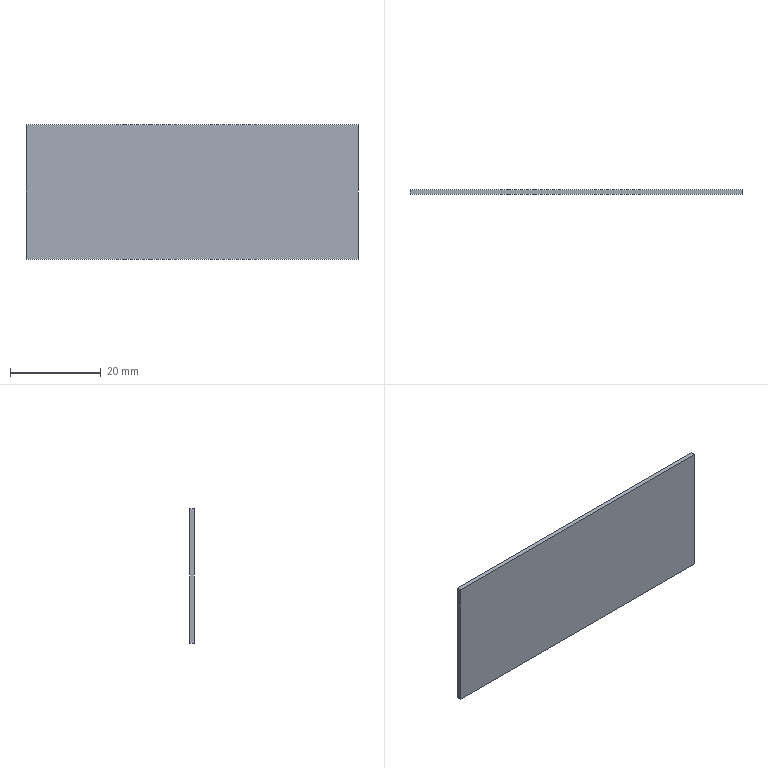Part | STEP file | 09-22 Inlet side seal plate 2 | 1 solid | 6 faces | box 73 x 1 x 29.5 mm | volume 2153 mm3 | plane 6
STEP:
#1=CARTESIAN_POINT('',(0.,0.,0.));
#2=DIRECTION('',(0.,0.,1.));
#3=DIRECTION('',(1.,0.,0.));
#4=AXIS2_PLACEMENT_3D('',#1,#2,#3);
#5=CARTESIAN_POINT('',(73.,0.,0.));
#6=VERTEX_POINT('',#5);
#7=CARTESIAN_POINT('',(0.,0.,0.));
#8=VERTEX_POINT('',#7);
#9=CARTESIAN_POINT('',(36.5,0.,0.));
#10=DIRECTION('',(-1.,0.,0.));
#11=VECTOR('',#10,1.);
#12=LINE('',#9,#11);
#13=CARTESIAN_POINT('',(73.,0.,0.));
#14=DIRECTION('',(0.,0.,-1.));
#15=DIRECTION('',(-1.,0.,0.));
#16=AXIS2_PLACEMENT_3D('',#13,#14,#15);
#17=PLANE('',#16);
#18=CARTESIAN_POINT('',(36.5,0.));
#19=DIRECTION('',(1.,0.));
#20=VECTOR('',#19,1.);
#21=LINE('',#18,#20);
#22=(GEOMETRIC_REPRESENTATION_CONTEXT(2)PARAMETRIC_REPRESENTATION_CONTEXT()REPRESENTATION_CONTEXT('',''));
#23=DEFINITIONAL_REPRESENTATION('',(#21),#22);
#24=PCURVE('',#17,#23);
#25=CARTESIAN_POINT('',(0.,0.,-29.5));
#26=DIRECTION('',(0.,1.,0.));
#27=DIRECTION('',(0.,0.,1.));
#28=AXIS2_PLACEMENT_3D('',#25,#26,#27);
#29=PLANE('',#28);
#30=CARTESIAN_POINT('',(29.5,36.5));
#31=DIRECTION('',(0.,-1.));
#32=VECTOR('',#31,1.);
#33=LINE('',#30,#32);
#34=(GEOMETRIC_REPRESENTATION_CONTEXT(2)PARAMETRIC_REPRESENTATION_CONTEXT()REPRESENTATION_CONTEXT('',''));
#35=DEFINITIONAL_REPRESENTATION('',(#33),#34);
#36=PCURVE('',#29,#35);
#37=SURFACE_CURVE('',#12,(#24,#36),.PCURVE_S1.);
#38=EDGE_CURVE('',#6,#8,#37,.T.);
#39=ORIENTED_EDGE('',*,*,#38,.F.);
#40=CARTESIAN_POINT('',(73.,1.,0.));
#41=VERTEX_POINT('',#40);
#42=CARTESIAN_POINT('',(73.,0.5,0.));
#43=DIRECTION('',(0.,1.,0.));
#44=VECTOR('',#43,1.);
#45=LINE('',#42,#44);
#46=CARTESIAN_POINT('',(0.,0.5));
#47=DIRECTION('',(0.,1.));
#48=VECTOR('',#47,1.);
#49=LINE('',#46,#48);
#50=(GEOMETRIC_REPRESENTATION_CONTEXT(2)PARAMETRIC_REPRESENTATION_CONTEXT()REPRESENTATION_CONTEXT('',''));
#51=DEFINITIONAL_REPRESENTATION('',(#49),#50);
#52=PCURVE('',#17,#51);
#53=CARTESIAN_POINT('',(73.,0.,-29.5));
#54=DIRECTION('',(-1.,0.,0.));
#55=DIRECTION('',(0.,0.,1.));
#56=AXIS2_PLACEMENT_3D('',#53,#54,#55);
#57=PLANE('',#56);
#58=CARTESIAN_POINT('',(29.5,0.5));
#59=DIRECTION('',(0.,1.));
#60=VECTOR('',#59,1.);
#61=LINE('',#58,#60);
#62=(GEOMETRIC_REPRESENTATION_CONTEXT(2)PARAMETRIC_REPRESENTATION_CONTEXT()REPRESENTATION_CONTEXT('',''));
#63=DEFINITIONAL_REPRESENTATION('',(#61),#62);
#64=PCURVE('',#57,#63);
#65=SURFACE_CURVE('',#45,(#52,#64),.PCURVE_S1.);
#66=EDGE_CURVE('',#6,#41,#65,.T.);
#67=ORIENTED_EDGE('',*,*,#66,.T.);
#68=CARTESIAN_POINT('',(0.,1.,0.));
#69=VERTEX_POINT('',#68);
#70=CARTESIAN_POINT('',(36.5,1.,0.));
#71=DIRECTION('',(1.,0.,0.));
#72=VECTOR('',#71,1.);
#73=LINE('',#70,#72);
#74=CARTESIAN_POINT('',(36.5,1.));
#75=DIRECTION('',(-1.,0.));
#76=VECTOR('',#75,1.);
#77=LINE('',#74,#76);
#78=(GEOMETRIC_REPRESENTATION_CONTEXT(2)PARAMETRIC_REPRESENTATION_CONTEXT()REPRESENTATION_CONTEXT('',''));
#79=DEFINITIONAL_REPRESENTATION('',(#77),#78);
#80=PCURVE('',#17,#79);
#81=CARTESIAN_POINT('',(0.,1.,0.));
#82=DIRECTION('',(0.,-1.,0.));
#83=DIRECTION('',(0.,0.,-1.));
#84=AXIS2_PLACEMENT_3D('',#81,#82,#83);
#85=PLANE('',#84);
#86=CARTESIAN_POINT('',(0.,36.5));
#87=DIRECTION('',(0.,1.));
#88=VECTOR('',#87,1.);
#89=LINE('',#86,#88);
#90=(GEOMETRIC_REPRESENTATION_CONTEXT(2)PARAMETRIC_REPRESENTATION_CONTEXT()REPRESENTATION_CONTEXT('',''));
#91=DEFINITIONAL_REPRESENTATION('',(#89),#90);
#92=PCURVE('',#85,#91);
#93=SURFACE_CURVE('',#73,(#80,#92),.PCURVE_S1.);
#94=EDGE_CURVE('',#69,#41,#93,.T.);
#95=ORIENTED_EDGE('',*,*,#94,.F.);
#96=CARTESIAN_POINT('',(0.,0.5,0.));
#97=DIRECTION('',(0.,1.,0.));
#98=VECTOR('',#97,1.);
#99=LINE('',#96,#98);
#100=CARTESIAN_POINT('',(73.,0.5));
#101=DIRECTION('',(0.,1.));
#102=VECTOR('',#101,1.);
#103=LINE('',#100,#102);
#104=(GEOMETRIC_REPRESENTATION_CONTEXT(2)PARAMETRIC_REPRESENTATION_CONTEXT()REPRESENTATION_CONTEXT('',''));
#105=DEFINITIONAL_REPRESENTATION('',(#103),#104);
#106=PCURVE('',#17,#105);
#107=CARTESIAN_POINT('',(0.,0.,-29.5));
#108=DIRECTION('',(-1.,0.,0.));
#109=DIRECTION('',(0.,0.,1.));
#110=AXIS2_PLACEMENT_3D('',#107,#108,#109);
#111=PLANE('',#110);
#112=CARTESIAN_POINT('',(29.5,0.5));
#113=DIRECTION('',(0.,1.));
#114=VECTOR('',#113,1.);
#115=LINE('',#112,#114);
#116=(GEOMETRIC_REPRESENTATION_CONTEXT(2)PARAMETRIC_REPRESENTATION_CONTEXT()REPRESENTATION_CONTEXT('',''));
#117=DEFINITIONAL_REPRESENTATION('',(#115),#116);
#118=PCURVE('',#111,#117);
#119=SURFACE_CURVE('',#99,(#106,#118),.PCURVE_S1.);
#120=EDGE_CURVE('',#8,#69,#119,.T.);
#121=ORIENTED_EDGE('',*,*,#120,.F.);
#122=EDGE_LOOP('',(#39,#67,#95,#121));
#123=FACE_BOUND('',#122,.T.);
#124=ADVANCED_FACE('',(#123),#17,.F.);
#125=CARTESIAN_POINT('',(73.,0.,-29.5));
#126=VERTEX_POINT('',#125);
#127=CARTESIAN_POINT('',(0.,0.,-29.5));
#128=VERTEX_POINT('',#127);
#129=CARTESIAN_POINT('',(36.5,0.,-29.5));
#130=DIRECTION('',(-1.,0.,0.));
#131=VECTOR('',#130,1.);
#132=LINE('',#129,#131);
#133=CARTESIAN_POINT('',(0.,36.5));
#134=DIRECTION('',(0.,-1.));
#135=VECTOR('',#134,1.);
#136=LINE('',#133,#135);
#137=(GEOMETRIC_REPRESENTATION_CONTEXT(2)PARAMETRIC_REPRESENTATION_CONTEXT()REPRESENTATION_CONTEXT('',''));
#138=DEFINITIONAL_REPRESENTATION('',(#136),#137);
#139=PCURVE('',#29,#138);
#140=CARTESIAN_POINT('',(0.,0.,-29.5));
#141=DIRECTION('',(0.,0.,1.));
#142=DIRECTION('',(1.,0.,0.));
#143=AXIS2_PLACEMENT_3D('',#140,#141,#142);
#144=PLANE('',#143);
#145=CARTESIAN_POINT('',(36.5,0.));
#146=DIRECTION('',(-1.,0.));
#147=VECTOR('',#146,1.);
#148=LINE('',#145,#147);
#149=(GEOMETRIC_REPRESENTATION_CONTEXT(2)PARAMETRIC_REPRESENTATION_CONTEXT()REPRESENTATION_CONTEXT('',''));
#150=DEFINITIONAL_REPRESENTATION('',(#148),#149);
#151=PCURVE('',#144,#150);
#152=SURFACE_CURVE('',#132,(#139,#151),.PCURVE_S1.);
#153=EDGE_CURVE('',#126,#128,#152,.T.);
#154=ORIENTED_EDGE('',*,*,#153,.F.);
#155=CARTESIAN_POINT('',(73.,0.,-14.75));
#156=DIRECTION('',(0.,0.,-1.));
#157=VECTOR('',#156,1.);
#158=LINE('',#155,#157);
#159=CARTESIAN_POINT('',(14.75,73.));
#160=DIRECTION('',(-1.,0.));
#161=VECTOR('',#160,1.);
#162=LINE('',#159,#161);
#163=(GEOMETRIC_REPRESENTATION_CONTEXT(2)PARAMETRIC_REPRESENTATION_CONTEXT()REPRESENTATION_CONTEXT('',''));
#164=DEFINITIONAL_REPRESENTATION('',(#162),#163);
#165=PCURVE('',#29,#164);
#166=CARTESIAN_POINT('',(14.75,0.));
#167=DIRECTION('',(-1.,0.));
#168=VECTOR('',#167,1.);
#169=LINE('',#166,#168);
#170=(GEOMETRIC_REPRESENTATION_CONTEXT(2)PARAMETRIC_REPRESENTATION_CONTEXT()REPRESENTATION_CONTEXT('',''));
#171=DEFINITIONAL_REPRESENTATION('',(#169),#170);
#172=PCURVE('',#57,#171);
#173=SURFACE_CURVE('',#158,(#165,#172),.PCURVE_S1.);
#174=EDGE_CURVE('',#6,#126,#173,.T.);
#175=ORIENTED_EDGE('',*,*,#174,.F.);
#176=ORIENTED_EDGE('',*,*,#38,.T.);
#177=CARTESIAN_POINT('',(0.,0.,-14.75));
#178=DIRECTION('',(0.,0.,1.));
#179=VECTOR('',#178,1.);
#180=LINE('',#177,#179);
#181=CARTESIAN_POINT('',(14.75,0.));
#182=DIRECTION('',(1.,0.));
#183=VECTOR('',#182,1.);
#184=LINE('',#181,#183);
#185=(GEOMETRIC_REPRESENTATION_CONTEXT(2)PARAMETRIC_REPRESENTATION_CONTEXT()REPRESENTATION_CONTEXT('',''));
#186=DEFINITIONAL_REPRESENTATION('',(#184),#185);
#187=PCURVE('',#29,#186);
#188=CARTESIAN_POINT('',(14.75,0.));
#189=DIRECTION('',(1.,0.));
#190=VECTOR('',#189,1.);
#191=LINE('',#188,#190);
#192=(GEOMETRIC_REPRESENTATION_CONTEXT(2)PARAMETRIC_REPRESENTATION_CONTEXT()REPRESENTATION_CONTEXT('',''));
#193=DEFINITIONAL_REPRESENTATION('',(#191),#192);
#194=PCURVE('',#111,#193);
#195=SURFACE_CURVE('',#180,(#187,#194),.PCURVE_S1.);
#196=EDGE_CURVE('',#128,#8,#195,.T.);
#197=ORIENTED_EDGE('',*,*,#196,.F.);
#198=EDGE_LOOP('',(#154,#175,#176,#197));
#199=FACE_BOUND('',#198,.T.);
#200=ADVANCED_FACE('',(#199),#29,.F.);
#201=ORIENTED_EDGE('',*,*,#94,.T.);
#202=CARTESIAN_POINT('',(73.,1.,-29.5));
#203=VERTEX_POINT('',#202);
#204=CARTESIAN_POINT('',(73.,1.,-14.75));
#205=DIRECTION('',(0.,0.,1.));
#206=VECTOR('',#205,1.);
#207=LINE('',#204,#206);
#208=CARTESIAN_POINT('',(14.75,73.));
#209=DIRECTION('',(-1.,0.));
#210=VECTOR('',#209,1.);
#211=LINE('',#208,#210);
#212=(GEOMETRIC_REPRESENTATION_CONTEXT(2)PARAMETRIC_REPRESENTATION_CONTEXT()REPRESENTATION_CONTEXT('',''));
#213=DEFINITIONAL_REPRESENTATION('',(#211),#212);
#214=PCURVE('',#85,#213);
#215=CARTESIAN_POINT('',(14.75,1.));
#216=DIRECTION('',(1.,0.));
#217=VECTOR('',#216,1.);
#218=LINE('',#215,#217);
#219=(GEOMETRIC_REPRESENTATION_CONTEXT(2)PARAMETRIC_REPRESENTATION_CONTEXT()REPRESENTATION_CONTEXT('',''));
#220=DEFINITIONAL_REPRESENTATION('',(#218),#219);
#221=PCURVE('',#57,#220);
#222=SURFACE_CURVE('',#207,(#214,#221),.PCURVE_S1.);
#223=EDGE_CURVE('',#203,#41,#222,.T.);
#224=ORIENTED_EDGE('',*,*,#223,.F.);
#225=CARTESIAN_POINT('',(0.,1.,-29.5));
#226=VERTEX_POINT('',#225);
#227=CARTESIAN_POINT('',(36.5,1.,-29.5));
#228=DIRECTION('',(1.,0.,0.));
#229=VECTOR('',#228,1.);
#230=LINE('',#227,#229);
#231=CARTESIAN_POINT('',(29.5,36.5));
#232=DIRECTION('',(0.,1.));
#233=VECTOR('',#232,1.);
#234=LINE('',#231,#233);
#235=(GEOMETRIC_REPRESENTATION_CONTEXT(2)PARAMETRIC_REPRESENTATION_CONTEXT()REPRESENTATION_CONTEXT('',''));
#236=DEFINITIONAL_REPRESENTATION('',(#234),#235);
#237=PCURVE('',#85,#236);
#238=CARTESIAN_POINT('',(36.5,1.));
#239=DIRECTION('',(1.,0.));
#240=VECTOR('',#239,1.);
#241=LINE('',#238,#240);
#242=(GEOMETRIC_REPRESENTATION_CONTEXT(2)PARAMETRIC_REPRESENTATION_CONTEXT()REPRESENTATION_CONTEXT('',''));
#243=DEFINITIONAL_REPRESENTATION('',(#241),#242);
#244=PCURVE('',#144,#243);
#245=SURFACE_CURVE('',#230,(#237,#244),.PCURVE_S1.);
#246=EDGE_CURVE('',#226,#203,#245,.T.);
#247=ORIENTED_EDGE('',*,*,#246,.F.);
#248=CARTESIAN_POINT('',(0.,1.,-14.75));
#249=DIRECTION('',(0.,0.,-1.));
#250=VECTOR('',#249,1.);
#251=LINE('',#248,#250);
#252=CARTESIAN_POINT('',(14.75,0.));
#253=DIRECTION('',(1.,0.));
#254=VECTOR('',#253,1.);
#255=LINE('',#252,#254);
#256=(GEOMETRIC_REPRESENTATION_CONTEXT(2)PARAMETRIC_REPRESENTATION_CONTEXT()REPRESENTATION_CONTEXT('',''));
#257=DEFINITIONAL_REPRESENTATION('',(#255),#256);
#258=PCURVE('',#85,#257);
#259=CARTESIAN_POINT('',(14.75,1.));
#260=DIRECTION('',(-1.,0.));
#261=VECTOR('',#260,1.);
#262=LINE('',#259,#261);
#263=(GEOMETRIC_REPRESENTATION_CONTEXT(2)PARAMETRIC_REPRESENTATION_CONTEXT()REPRESENTATION_CONTEXT('',''));
#264=DEFINITIONAL_REPRESENTATION('',(#262),#263);
#265=PCURVE('',#111,#264);
#266=SURFACE_CURVE('',#251,(#258,#265),.PCURVE_S1.);
#267=EDGE_CURVE('',#69,#226,#266,.T.);
#268=ORIENTED_EDGE('',*,*,#267,.F.);
#269=EDGE_LOOP('',(#201,#224,#247,#268));
#270=FACE_BOUND('',#269,.T.);
#271=ADVANCED_FACE('',(#270),#85,.F.);
#272=CARTESIAN_POINT('',(0.,0.5,-29.5));
#273=DIRECTION('',(0.,-1.,0.));
#274=VECTOR('',#273,1.);
#275=LINE('',#272,#274);
#276=CARTESIAN_POINT('',(0.,0.5));
#277=DIRECTION('',(0.,-1.));
#278=VECTOR('',#277,1.);
#279=LINE('',#276,#278);
#280=(GEOMETRIC_REPRESENTATION_CONTEXT(2)PARAMETRIC_REPRESENTATION_CONTEXT()REPRESENTATION_CONTEXT('',''));
#281=DEFINITIONAL_REPRESENTATION('',(#279),#280);
#282=PCURVE('',#111,#281);
#283=CARTESIAN_POINT('',(0.,0.5));
#284=DIRECTION('',(0.,-1.));
#285=VECTOR('',#284,1.);
#286=LINE('',#283,#285);
#287=(GEOMETRIC_REPRESENTATION_CONTEXT(2)PARAMETRIC_REPRESENTATION_CONTEXT()REPRESENTATION_CONTEXT('',''));
#288=DEFINITIONAL_REPRESENTATION('',(#286),#287);
#289=PCURVE('',#144,#288);
#290=SURFACE_CURVE('',#275,(#282,#289),.PCURVE_S1.);
#291=EDGE_CURVE('',#226,#128,#290,.T.);
#292=ORIENTED_EDGE('',*,*,#291,.T.);
#293=ORIENTED_EDGE('',*,*,#196,.T.);
#294=ORIENTED_EDGE('',*,*,#120,.T.);
#295=ORIENTED_EDGE('',*,*,#267,.T.);
#296=EDGE_LOOP('',(#292,#293,#294,#295));
#297=FACE_BOUND('',#296,.T.);
#298=ADVANCED_FACE('',(#297),#111,.T.);
#299=ORIENTED_EDGE('',*,*,#246,.T.);
#300=CARTESIAN_POINT('',(73.,0.5,-29.5));
#301=DIRECTION('',(0.,1.,0.));
#302=VECTOR('',#301,1.);
#303=LINE('',#300,#302);
#304=CARTESIAN_POINT('',(73.,0.5));
#305=DIRECTION('',(0.,1.));
#306=VECTOR('',#305,1.);
#307=LINE('',#304,#306);
#308=(GEOMETRIC_REPRESENTATION_CONTEXT(2)PARAMETRIC_REPRESENTATION_CONTEXT()REPRESENTATION_CONTEXT('',''));
#309=DEFINITIONAL_REPRESENTATION('',(#307),#308);
#310=PCURVE('',#144,#309);
#311=CARTESIAN_POINT('',(0.,0.5));
#312=DIRECTION('',(0.,1.));
#313=VECTOR('',#312,1.);
#314=LINE('',#311,#313);
#315=(GEOMETRIC_REPRESENTATION_CONTEXT(2)PARAMETRIC_REPRESENTATION_CONTEXT()REPRESENTATION_CONTEXT('',''));
#316=DEFINITIONAL_REPRESENTATION('',(#314),#315);
#317=PCURVE('',#57,#316);
#318=SURFACE_CURVE('',#303,(#310,#317),.PCURVE_S1.);
#319=EDGE_CURVE('',#126,#203,#318,.T.);
#320=ORIENTED_EDGE('',*,*,#319,.F.);
#321=ORIENTED_EDGE('',*,*,#153,.T.);
#322=ORIENTED_EDGE('',*,*,#291,.F.);
#323=EDGE_LOOP('',(#299,#320,#321,#322));
#324=FACE_BOUND('',#323,.T.);
#325=ADVANCED_FACE('',(#324),#144,.F.);
#326=ORIENTED_EDGE('',*,*,#174,.T.);
#327=ORIENTED_EDGE('',*,*,#319,.T.);
#328=ORIENTED_EDGE('',*,*,#223,.T.);
#329=ORIENTED_EDGE('',*,*,#66,.F.);
#330=EDGE_LOOP('',(#326,#327,#328,#329));
#331=FACE_BOUND('',#330,.T.);
#332=ADVANCED_FACE('',(#331),#57,.F.);
#333=CLOSED_SHELL('',(#124,#200,#271,#298,#325,#332));
#334=MANIFOLD_SOLID_BREP('',#333);
#335=(LENGTH_UNIT()NAMED_UNIT(*)SI_UNIT(.MILLI.,.METRE.));
#336=UNCERTAINTY_MEASURE_WITH_UNIT(LENGTH_MEASURE(0.0000001),#335,'','');
#337=(NAMED_UNIT(*)PLANE_ANGLE_UNIT()SI_UNIT($,.RADIAN.));
#338=(NAMED_UNIT(*)SI_UNIT($,.STERADIAN.)SOLID_ANGLE_UNIT());
#339=(GEOMETRIC_REPRESENTATION_CONTEXT(3)GLOBAL_UNCERTAINTY_ASSIGNED_CONTEXT((#336))GLOBAL_UNIT_ASSIGNED_CONTEXT((#335,#337,#338))REPRESENTATION_CONTEXT('',''));
#340=ADVANCED_BREP_SHAPE_REPRESENTATION('',(#4,#334),#339);